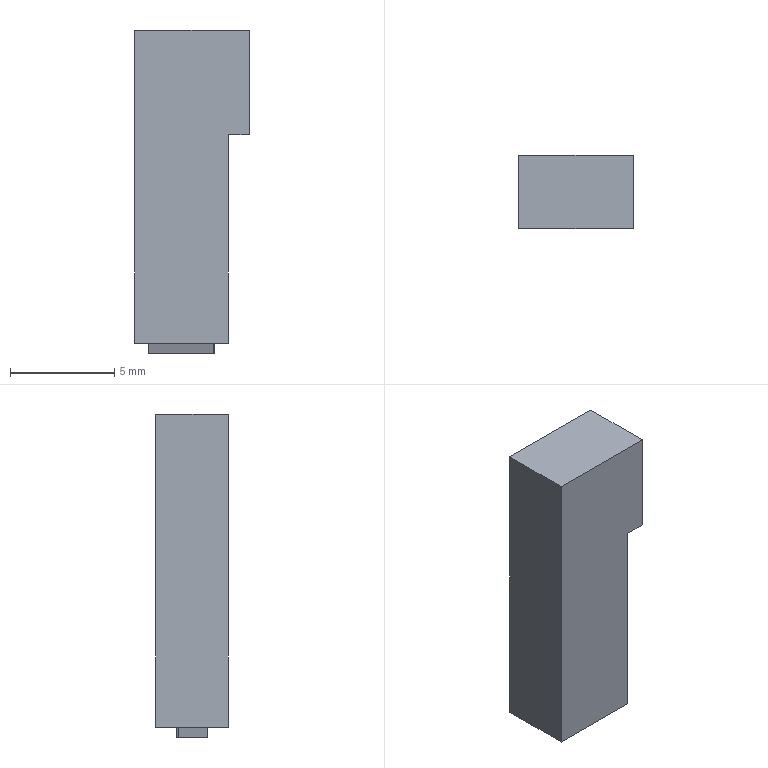Part | STEP file | gslz 2016.10.28-10_id1638_x_t | 1 solid | 13 faces | box 5.5 x 3.5 x 15.5 mm | volume 253.941 mm3 | plane 13
STEP:
#1=CARTESIAN_POINT('',(0.,0.,0.));
#2=DIRECTION('',(0.,0.,1.));
#3=DIRECTION('',(1.,0.,0.));
#4=AXIS2_PLACEMENT_3D('',#1,#2,#3);
#5=CARTESIAN_POINT('',(-688.56,94.749,15.));
#6=VERTEX_POINT('',#5);
#7=CARTESIAN_POINT('',(-694.06,94.749,15.));
#8=VERTEX_POINT('',#7);
#9=CARTESIAN_POINT('',(-691.31,94.749,15.));
#10=DIRECTION('',(-1.,0.000000055,0.));
#11=VECTOR('',#10,1.);
#12=LINE('',#9,#11);
#13=CARTESIAN_POINT('',(-694.06,94.749,15.));
#14=DIRECTION('',(-0.000000055,-1.,0.));
#15=DIRECTION('',(-1.,0.000000055,0.));
#16=AXIS2_PLACEMENT_3D('',#13,#14,#15);
#17=PLANE('',#16);
#18=CARTESIAN_POINT('',(-2.75,0.));
#19=DIRECTION('',(1.,0.));
#20=VECTOR('',#19,1.);
#21=LINE('',#18,#20);
#22=(GEOMETRIC_REPRESENTATION_CONTEXT(2)PARAMETRIC_REPRESENTATION_CONTEXT()REPRESENTATION_CONTEXT('',''));
#23=DEFINITIONAL_REPRESENTATION('',(#21),#22);
#24=PCURVE('',#17,#23);
#25=CARTESIAN_POINT('',(-694.06,96.499,15.));
#26=DIRECTION('',(0.,0.,1.));
#27=DIRECTION('',(1.,0.,0.));
#28=AXIS2_PLACEMENT_3D('',#25,#26,#27);
#29=PLANE('',#28);
#30=CARTESIAN_POINT('',(2.75,-1.75));
#31=DIRECTION('',(-1.,0.000000055));
#32=VECTOR('',#31,1.);
#33=LINE('',#30,#32);
#34=(GEOMETRIC_REPRESENTATION_CONTEXT(2)PARAMETRIC_REPRESENTATION_CONTEXT()REPRESENTATION_CONTEXT('',''));
#35=DEFINITIONAL_REPRESENTATION('',(#33),#34);
#36=PCURVE('',#29,#35);
#37=SURFACE_CURVE('',#12,(#24,#36),.PCURVE_S1.);
#38=EDGE_CURVE('',#6,#8,#37,.T.);
#39=ORIENTED_EDGE('',*,*,#38,.T.);
#40=CARTESIAN_POINT('',(-694.06,94.749,0.));
#41=VERTEX_POINT('',#40);
#42=CARTESIAN_POINT('',(-694.06,94.749,15.));
#43=DIRECTION('',(0.,0.,1.));
#44=VECTOR('',#43,1.);
#45=LINE('',#42,#44);
#46=CARTESIAN_POINT('',(0.,0.));
#47=DIRECTION('',(0.,-1.));
#48=VECTOR('',#47,1.);
#49=LINE('',#46,#48);
#50=(GEOMETRIC_REPRESENTATION_CONTEXT(2)PARAMETRIC_REPRESENTATION_CONTEXT()REPRESENTATION_CONTEXT('',''));
#51=DEFINITIONAL_REPRESENTATION('',(#49),#50);
#52=PCURVE('',#17,#51);
#53=CARTESIAN_POINT('',(-694.06,98.249,15.));
#54=DIRECTION('',(-1.,0.,0.));
#55=DIRECTION('',(0.,1.,0.));
#56=AXIS2_PLACEMENT_3D('',#53,#54,#55);
#57=PLANE('',#56);
#58=CARTESIAN_POINT('',(-3.5,0.));
#59=DIRECTION('',(0.,-1.));
#60=VECTOR('',#59,1.);
#61=LINE('',#58,#60);
#62=(GEOMETRIC_REPRESENTATION_CONTEXT(2)PARAMETRIC_REPRESENTATION_CONTEXT()REPRESENTATION_CONTEXT('',''));
#63=DEFINITIONAL_REPRESENTATION('',(#61),#62);
#64=PCURVE('',#57,#63);
#65=SURFACE_CURVE('',#45,(#52,#64),.PCURVE_S1.);
#66=EDGE_CURVE('',#41,#8,#65,.T.);
#67=ORIENTED_EDGE('',*,*,#66,.F.);
#68=CARTESIAN_POINT('',(-689.56,94.749,0.));
#69=VERTEX_POINT('',#68);
#70=CARTESIAN_POINT('',(-691.31,94.749,0.));
#71=DIRECTION('',(-1.,0.000000055,0.));
#72=VECTOR('',#71,1.);
#73=LINE('',#70,#72);
#74=CARTESIAN_POINT('',(-2.75,15.));
#75=DIRECTION('',(1.,0.));
#76=VECTOR('',#75,1.);
#77=LINE('',#74,#76);
#78=(GEOMETRIC_REPRESENTATION_CONTEXT(2)PARAMETRIC_REPRESENTATION_CONTEXT()REPRESENTATION_CONTEXT('',''));
#79=DEFINITIONAL_REPRESENTATION('',(#77),#78);
#80=PCURVE('',#17,#79);
#81=CARTESIAN_POINT('',(-694.06,96.499,0.));
#82=DIRECTION('',(0.,0.,1.));
#83=DIRECTION('',(1.,0.,0.));
#84=AXIS2_PLACEMENT_3D('',#81,#82,#83);
#85=PLANE('',#84);
#86=CARTESIAN_POINT('',(2.75,-1.75));
#87=DIRECTION('',(-1.,0.000000055));
#88=VECTOR('',#87,1.);
#89=LINE('',#86,#88);
#90=(GEOMETRIC_REPRESENTATION_CONTEXT(2)PARAMETRIC_REPRESENTATION_CONTEXT()REPRESENTATION_CONTEXT('',''));
#91=DEFINITIONAL_REPRESENTATION('',(#89),#90);
#92=PCURVE('',#85,#91);
#93=SURFACE_CURVE('',#73,(#80,#92),.PCURVE_S1.);
#94=EDGE_CURVE('',#69,#41,#93,.T.);
#95=ORIENTED_EDGE('',*,*,#94,.F.);
#96=CARTESIAN_POINT('',(-689.56,94.749,10.));
#97=VERTEX_POINT('',#96);
#98=CARTESIAN_POINT('',(-689.56,94.749,15.));
#99=DIRECTION('',(0.,0.,-1.));
#100=VECTOR('',#99,1.);
#101=LINE('',#98,#100);
#102=CARTESIAN_POINT('',(-4.5,0.));
#103=DIRECTION('',(0.,1.));
#104=VECTOR('',#103,1.);
#105=LINE('',#102,#104);
#106=(GEOMETRIC_REPRESENTATION_CONTEXT(2)PARAMETRIC_REPRESENTATION_CONTEXT()REPRESENTATION_CONTEXT('',''));
#107=DEFINITIONAL_REPRESENTATION('',(#105),#106);
#108=PCURVE('',#17,#107);
#109=CARTESIAN_POINT('',(-689.56,96.499,7.5));
#110=DIRECTION('',(1.,0.,0.));
#111=DIRECTION('',(0.,0.,-1.));
#112=AXIS2_PLACEMENT_3D('',#109,#110,#111);
#113=PLANE('',#112);
#114=CARTESIAN_POINT('',(-7.5,-1.75));
#115=DIRECTION('',(1.,0.));
#116=VECTOR('',#115,1.);
#117=LINE('',#114,#116);
#118=(GEOMETRIC_REPRESENTATION_CONTEXT(2)PARAMETRIC_REPRESENTATION_CONTEXT()REPRESENTATION_CONTEXT('',''));
#119=DEFINITIONAL_REPRESENTATION('',(#117),#118);
#120=PCURVE('',#113,#119);
#121=SURFACE_CURVE('',#101,(#108,#120),.PCURVE_S1.);
#122=EDGE_CURVE('',#97,#69,#121,.T.);
#123=ORIENTED_EDGE('',*,*,#122,.F.);
#124=CARTESIAN_POINT('',(-688.56,94.749,10.));
#125=VERTEX_POINT('',#124);
#126=CARTESIAN_POINT('',(-694.06,94.749,10.));
#127=DIRECTION('',(-1.,0.000000055,0.));
#128=VECTOR('',#127,1.);
#129=LINE('',#126,#128);
#130=CARTESIAN_POINT('',(0.,5.));
#131=DIRECTION('',(1.,0.));
#132=VECTOR('',#131,1.);
#133=LINE('',#130,#132);
#134=(GEOMETRIC_REPRESENTATION_CONTEXT(2)PARAMETRIC_REPRESENTATION_CONTEXT()REPRESENTATION_CONTEXT('',''));
#135=DEFINITIONAL_REPRESENTATION('',(#133),#134);
#136=PCURVE('',#17,#135);
#137=CARTESIAN_POINT('',(-694.06,96.499,10.));
#138=DIRECTION('',(0.,0.,1.));
#139=DIRECTION('',(1.,0.,0.));
#140=AXIS2_PLACEMENT_3D('',#137,#138,#139);
#141=PLANE('',#140);
#142=CARTESIAN_POINT('',(0.,-1.75));
#143=DIRECTION('',(-1.,0.000000055));
#144=VECTOR('',#143,1.);
#145=LINE('',#142,#144);
#146=(GEOMETRIC_REPRESENTATION_CONTEXT(2)PARAMETRIC_REPRESENTATION_CONTEXT()REPRESENTATION_CONTEXT('',''));
#147=DEFINITIONAL_REPRESENTATION('',(#145),#146);
#148=PCURVE('',#141,#147);
#149=SURFACE_CURVE('',#129,(#136,#148),.PCURVE_S1.);
#150=EDGE_CURVE('',#125,#97,#149,.T.);
#151=ORIENTED_EDGE('',*,*,#150,.F.);
#152=CARTESIAN_POINT('',(-688.56,94.749,15.));
#153=DIRECTION('',(0.,0.,1.));
#154=VECTOR('',#153,1.);
#155=LINE('',#152,#154);
#156=CARTESIAN_POINT('',(-5.5,0.));
#157=DIRECTION('',(0.,-1.));
#158=VECTOR('',#157,1.);
#159=LINE('',#156,#158);
#160=(GEOMETRIC_REPRESENTATION_CONTEXT(2)PARAMETRIC_REPRESENTATION_CONTEXT()REPRESENTATION_CONTEXT('',''));
#161=DEFINITIONAL_REPRESENTATION('',(#159),#160);
#162=PCURVE('',#17,#161);
#163=CARTESIAN_POINT('',(-688.56,94.749,15.));
#164=DIRECTION('',(1.,0.,0.));
#165=DIRECTION('',(0.,-1.,0.));
#166=AXIS2_PLACEMENT_3D('',#163,#164,#165);
#167=PLANE('',#166);
#168=CARTESIAN_POINT('',(0.,0.));
#169=DIRECTION('',(0.,-1.));
#170=VECTOR('',#169,1.);
#171=LINE('',#168,#170);
#172=(GEOMETRIC_REPRESENTATION_CONTEXT(2)PARAMETRIC_REPRESENTATION_CONTEXT()REPRESENTATION_CONTEXT('',''));
#173=DEFINITIONAL_REPRESENTATION('',(#171),#172);
#174=PCURVE('',#167,#173);
#175=SURFACE_CURVE('',#155,(#162,#174),.PCURVE_S1.);
#176=EDGE_CURVE('',#125,#6,#175,.T.);
#177=ORIENTED_EDGE('',*,*,#176,.T.);
#178=EDGE_LOOP('',(#39,#67,#95,#123,#151,#177));
#179=FACE_BOUND('',#178,.T.);
#180=ADVANCED_FACE('',(#179),#17,.T.);
#181=CARTESIAN_POINT('',(-694.06,98.249,0.));
#182=VERTEX_POINT('',#181);
#183=CARTESIAN_POINT('',(-689.56,98.249,0.));
#184=VERTEX_POINT('',#183);
#185=CARTESIAN_POINT('',(-691.31,98.249,0.));
#186=DIRECTION('',(1.,-0.000000055,0.));
#187=VECTOR('',#186,1.);
#188=LINE('',#185,#187);
#189=CARTESIAN_POINT('',(-688.56,98.249,15.));
#190=DIRECTION('',(0.000000055,1.,0.));
#191=DIRECTION('',(1.,-0.000000055,0.));
#192=AXIS2_PLACEMENT_3D('',#189,#190,#191);
#193=PLANE('',#192);
#194=CARTESIAN_POINT('',(-2.75,15.));
#195=DIRECTION('',(1.,0.));
#196=VECTOR('',#195,1.);
#197=LINE('',#194,#196);
#198=(GEOMETRIC_REPRESENTATION_CONTEXT(2)PARAMETRIC_REPRESENTATION_CONTEXT()REPRESENTATION_CONTEXT('',''));
#199=DEFINITIONAL_REPRESENTATION('',(#197),#198);
#200=PCURVE('',#193,#199);
#201=CARTESIAN_POINT('',(2.75,1.75));
#202=DIRECTION('',(1.,-0.000000055));
#203=VECTOR('',#202,1.);
#204=LINE('',#201,#203);
#205=(GEOMETRIC_REPRESENTATION_CONTEXT(2)PARAMETRIC_REPRESENTATION_CONTEXT()REPRESENTATION_CONTEXT('',''));
#206=DEFINITIONAL_REPRESENTATION('',(#204),#205);
#207=PCURVE('',#85,#206);
#208=SURFACE_CURVE('',#188,(#200,#207),.PCURVE_S1.);
#209=EDGE_CURVE('',#182,#184,#208,.T.);
#210=ORIENTED_EDGE('',*,*,#209,.F.);
#211=CARTESIAN_POINT('',(-694.06,98.249,15.));
#212=VERTEX_POINT('',#211);
#213=CARTESIAN_POINT('',(-694.06,98.249,15.));
#214=DIRECTION('',(0.,0.,1.));
#215=VECTOR('',#214,1.);
#216=LINE('',#213,#215);
#217=CARTESIAN_POINT('',(-5.5,0.));
#218=DIRECTION('',(0.,-1.));
#219=VECTOR('',#218,1.);
#220=LINE('',#217,#219);
#221=(GEOMETRIC_REPRESENTATION_CONTEXT(2)PARAMETRIC_REPRESENTATION_CONTEXT()REPRESENTATION_CONTEXT('',''));
#222=DEFINITIONAL_REPRESENTATION('',(#220),#221);
#223=PCURVE('',#193,#222);
#224=CARTESIAN_POINT('',(0.,0.));
#225=DIRECTION('',(0.,-1.));
#226=VECTOR('',#225,1.);
#227=LINE('',#224,#226);
#228=(GEOMETRIC_REPRESENTATION_CONTEXT(2)PARAMETRIC_REPRESENTATION_CONTEXT()REPRESENTATION_CONTEXT('',''));
#229=DEFINITIONAL_REPRESENTATION('',(#227),#228);
#230=PCURVE('',#57,#229);
#231=SURFACE_CURVE('',#216,(#223,#230),.PCURVE_S1.);
#232=EDGE_CURVE('',#182,#212,#231,.T.);
#233=ORIENTED_EDGE('',*,*,#232,.T.);
#234=CARTESIAN_POINT('',(-688.56,98.249,15.));
#235=VERTEX_POINT('',#234);
#236=CARTESIAN_POINT('',(-691.31,98.249,15.));
#237=DIRECTION('',(1.,-0.000000055,0.));
#238=VECTOR('',#237,1.);
#239=LINE('',#236,#238);
#240=CARTESIAN_POINT('',(-2.75,0.));
#241=DIRECTION('',(1.,0.));
#242=VECTOR('',#241,1.);
#243=LINE('',#240,#242);
#244=(GEOMETRIC_REPRESENTATION_CONTEXT(2)PARAMETRIC_REPRESENTATION_CONTEXT()REPRESENTATION_CONTEXT('',''));
#245=DEFINITIONAL_REPRESENTATION('',(#243),#244);
#246=PCURVE('',#193,#245);
#247=CARTESIAN_POINT('',(2.75,1.75));
#248=DIRECTION('',(1.,-0.000000055));
#249=VECTOR('',#248,1.);
#250=LINE('',#247,#249);
#251=(GEOMETRIC_REPRESENTATION_CONTEXT(2)PARAMETRIC_REPRESENTATION_CONTEXT()REPRESENTATION_CONTEXT('',''));
#252=DEFINITIONAL_REPRESENTATION('',(#250),#251);
#253=PCURVE('',#29,#252);
#254=SURFACE_CURVE('',#239,(#246,#253),.PCURVE_S1.);
#255=EDGE_CURVE('',#212,#235,#254,.T.);
#256=ORIENTED_EDGE('',*,*,#255,.T.);
#257=CARTESIAN_POINT('',(-688.56,98.249,10.));
#258=VERTEX_POINT('',#257);
#259=CARTESIAN_POINT('',(-688.56,98.249,15.));
#260=DIRECTION('',(0.,0.,1.));
#261=VECTOR('',#260,1.);
#262=LINE('',#259,#261);
#263=CARTESIAN_POINT('',(0.,0.));
#264=DIRECTION('',(0.,-1.));
#265=VECTOR('',#264,1.);
#266=LINE('',#263,#265);
#267=(GEOMETRIC_REPRESENTATION_CONTEXT(2)PARAMETRIC_REPRESENTATION_CONTEXT()REPRESENTATION_CONTEXT('',''));
#268=DEFINITIONAL_REPRESENTATION('',(#266),#267);
#269=PCURVE('',#193,#268);
#270=CARTESIAN_POINT('',(-3.5,0.));
#271=DIRECTION('',(0.,-1.));
#272=VECTOR('',#271,1.);
#273=LINE('',#270,#272);
#274=(GEOMETRIC_REPRESENTATION_CONTEXT(2)PARAMETRIC_REPRESENTATION_CONTEXT()REPRESENTATION_CONTEXT('',''));
#275=DEFINITIONAL_REPRESENTATION('',(#273),#274);
#276=PCURVE('',#167,#275);
#277=SURFACE_CURVE('',#262,(#269,#276),.PCURVE_S1.);
#278=EDGE_CURVE('',#258,#235,#277,.T.);
#279=ORIENTED_EDGE('',*,*,#278,.F.);
#280=CARTESIAN_POINT('',(-689.56,98.249,10.));
#281=VERTEX_POINT('',#280);
#282=CARTESIAN_POINT('',(-688.56,98.249,10.));
#283=DIRECTION('',(1.,-0.000000055,0.));
#284=VECTOR('',#283,1.);
#285=LINE('',#282,#284);
#286=CARTESIAN_POINT('',(0.,5.));
#287=DIRECTION('',(1.,0.));
#288=VECTOR('',#287,1.);
#289=LINE('',#286,#288);
#290=(GEOMETRIC_REPRESENTATION_CONTEXT(2)PARAMETRIC_REPRESENTATION_CONTEXT()REPRESENTATION_CONTEXT('',''));
#291=DEFINITIONAL_REPRESENTATION('',(#289),#290);
#292=PCURVE('',#193,#291);
#293=CARTESIAN_POINT('',(5.5,1.75));
#294=DIRECTION('',(1.,-0.000000055));
#295=VECTOR('',#294,1.);
#296=LINE('',#293,#295);
#297=(GEOMETRIC_REPRESENTATION_CONTEXT(2)PARAMETRIC_REPRESENTATION_CONTEXT()REPRESENTATION_CONTEXT('',''));
#298=DEFINITIONAL_REPRESENTATION('',(#296),#297);
#299=PCURVE('',#141,#298);
#300=SURFACE_CURVE('',#285,(#292,#299),.PCURVE_S1.);
#301=EDGE_CURVE('',#281,#258,#300,.T.);
#302=ORIENTED_EDGE('',*,*,#301,.F.);
#303=CARTESIAN_POINT('',(-689.56,98.249,15.));
#304=DIRECTION('',(0.,0.,1.));
#305=VECTOR('',#304,1.);
#306=LINE('',#303,#305);
#307=CARTESIAN_POINT('',(-1.,0.));
#308=DIRECTION('',(0.,-1.));
#309=VECTOR('',#308,1.);
#310=LINE('',#307,#309);
#311=(GEOMETRIC_REPRESENTATION_CONTEXT(2)PARAMETRIC_REPRESENTATION_CONTEXT()REPRESENTATION_CONTEXT('',''));
#312=DEFINITIONAL_REPRESENTATION('',(#310),#311);
#313=PCURVE('',#193,#312);
#314=CARTESIAN_POINT('',(-7.5,1.75));
#315=DIRECTION('',(-1.,0.));
#316=VECTOR('',#315,1.);
#317=LINE('',#314,#316);
#318=(GEOMETRIC_REPRESENTATION_CONTEXT(2)PARAMETRIC_REPRESENTATION_CONTEXT()REPRESENTATION_CONTEXT('',''));
#319=DEFINITIONAL_REPRESENTATION('',(#317),#318);
#320=PCURVE('',#113,#319);
#321=SURFACE_CURVE('',#306,(#313,#320),.PCURVE_S1.);
#322=EDGE_CURVE('',#184,#281,#321,.T.);
#323=ORIENTED_EDGE('',*,*,#322,.F.);
#324=EDGE_LOOP('',(#210,#233,#256,#279,#302,#323));
#325=FACE_BOUND('',#324,.T.);
#326=ADVANCED_FACE('',(#325),#193,.T.);
#327=ORIENTED_EDGE('',*,*,#255,.F.);
#328=CARTESIAN_POINT('',(-694.06,96.499,15.));
#329=DIRECTION('',(0.,1.,0.));
#330=VECTOR('',#329,1.);
#331=LINE('',#328,#330);
#332=CARTESIAN_POINT('',(0.,0.));
#333=DIRECTION('',(0.,1.));
#334=VECTOR('',#333,1.);
#335=LINE('',#332,#334);
#336=(GEOMETRIC_REPRESENTATION_CONTEXT(2)PARAMETRIC_REPRESENTATION_CONTEXT()REPRESENTATION_CONTEXT('',''));
#337=DEFINITIONAL_REPRESENTATION('',(#335),#336);
#338=PCURVE('',#29,#337);
#339=CARTESIAN_POINT('',(-1.75,0.));
#340=DIRECTION('',(1.,0.));
#341=VECTOR('',#340,1.);
#342=LINE('',#339,#341);
#343=(GEOMETRIC_REPRESENTATION_CONTEXT(2)PARAMETRIC_REPRESENTATION_CONTEXT()REPRESENTATION_CONTEXT('',''));
#344=DEFINITIONAL_REPRESENTATION('',(#342),#343);
#345=PCURVE('',#57,#344);
#346=SURFACE_CURVE('',#331,(#338,#345),.PCURVE_S1.);
#347=EDGE_CURVE('',#8,#212,#346,.T.);
#348=ORIENTED_EDGE('',*,*,#347,.F.);
#349=ORIENTED_EDGE('',*,*,#38,.F.);
#350=CARTESIAN_POINT('',(-688.56,96.499,15.));
#351=DIRECTION('',(0.,-1.,0.));
#352=VECTOR('',#351,1.);
#353=LINE('',#350,#352);
#354=CARTESIAN_POINT('',(5.5,-0.000000303));
#355=DIRECTION('',(0.,-1.));
#356=VECTOR('',#355,1.);
#357=LINE('',#354,#356);
#358=(GEOMETRIC_REPRESENTATION_CONTEXT(2)PARAMETRIC_REPRESENTATION_CONTEXT()REPRESENTATION_CONTEXT('',''));
#359=DEFINITIONAL_REPRESENTATION('',(#357),#358);
#360=PCURVE('',#29,#359);
#361=CARTESIAN_POINT('',(-1.75,0.));
#362=DIRECTION('',(1.,0.));
#363=VECTOR('',#362,1.);
#364=LINE('',#361,#363);
#365=(GEOMETRIC_REPRESENTATION_CONTEXT(2)PARAMETRIC_REPRESENTATION_CONTEXT()REPRESENTATION_CONTEXT('',''));
#366=DEFINITIONAL_REPRESENTATION('',(#364),#365);
#367=PCURVE('',#167,#366);
#368=SURFACE_CURVE('',#353,(#360,#367),.PCURVE_S1.);
#369=EDGE_CURVE('',#235,#6,#368,.T.);
#370=ORIENTED_EDGE('',*,*,#369,.F.);
#371=EDGE_LOOP('',(#327,#348,#349,#370));
#372=FACE_BOUND('',#371,.T.);
#373=ADVANCED_FACE('',(#372),#29,.T.);
#374=CARTESIAN_POINT('',(-693.353,97.249,0.));
#375=VERTEX_POINT('',#374);
#376=CARTESIAN_POINT('',(-693.411,97.153,0.));
#377=VERTEX_POINT('',#376);
#378=CARTESIAN_POINT('',(-693.875,96.387,0.));
#379=DIRECTION('',(-0.5182,-0.8552,0.));
#380=VECTOR('',#379,1.);
#381=LINE('',#378,#380);
#382=CARTESIAN_POINT('',(0.185,-0.1121));
#383=DIRECTION('',(-0.5182,-0.8552));
#384=VECTOR('',#383,1.);
#385=LINE('',#382,#384);
#386=(GEOMETRIC_REPRESENTATION_CONTEXT(2)PARAMETRIC_REPRESENTATION_CONTEXT()REPRESENTATION_CONTEXT('',''));
#387=DEFINITIONAL_REPRESENTATION('',(#385),#386);
#388=PCURVE('',#85,#387);
#389=CARTESIAN_POINT('',(-693.411,97.153,-0.5));
#390=DIRECTION('',(-0.8552,0.5182,0.));
#391=DIRECTION('',(0.5182,0.8552,0.));
#392=AXIS2_PLACEMENT_3D('',#389,#390,#391);
#393=PLANE('',#392);
#394=CARTESIAN_POINT('',(-0.8956,-0.5));
#395=DIRECTION('',(-1.,0.));
#396=VECTOR('',#395,1.);
#397=LINE('',#394,#396);
#398=(GEOMETRIC_REPRESENTATION_CONTEXT(2)PARAMETRIC_REPRESENTATION_CONTEXT()REPRESENTATION_CONTEXT('',''));
#399=DEFINITIONAL_REPRESENTATION('',(#397),#398);
#400=PCURVE('',#393,#399);
#401=SURFACE_CURVE('',#381,(#388,#400),.PCURVE_S1.);
#402=EDGE_CURVE('',#375,#377,#401,.T.);
#403=ORIENTED_EDGE('',*,*,#402,.T.);
#404=CARTESIAN_POINT('',(-690.282,95.749,0.));
#405=VERTEX_POINT('',#404);
#406=CARTESIAN_POINT('',(-693.707,97.286,0.));
#407=DIRECTION('',(0.9123,-0.4094,0.));
#408=VECTOR('',#407,1.);
#409=LINE('',#406,#408);
#410=CARTESIAN_POINT('',(0.353,0.7867));
#411=DIRECTION('',(0.9123,-0.4094));
#412=VECTOR('',#411,1.);
#413=LINE('',#410,#412);
#414=(GEOMETRIC_REPRESENTATION_CONTEXT(2)PARAMETRIC_REPRESENTATION_CONTEXT()REPRESENTATION_CONTEXT('',''));
#415=DEFINITIONAL_REPRESENTATION('',(#413),#414);
#416=PCURVE('',#85,#415);
#417=CARTESIAN_POINT('',(-690.282,95.749,-0.5));
#418=DIRECTION('',(-0.4094,-0.9123,0.));
#419=DIRECTION('',(-0.9123,0.4094,0.));
#420=AXIS2_PLACEMENT_3D('',#417,#418,#419);
#421=PLANE('',#420);
#422=CARTESIAN_POINT('',(3.754,-0.5));
#423=DIRECTION('',(-1.,0.));
#424=VECTOR('',#423,1.);
#425=LINE('',#422,#424);
#426=(GEOMETRIC_REPRESENTATION_CONTEXT(2)PARAMETRIC_REPRESENTATION_CONTEXT()REPRESENTATION_CONTEXT('',''));
#427=DEFINITIONAL_REPRESENTATION('',(#425),#426);
#428=PCURVE('',#421,#427);
#429=SURFACE_CURVE('',#409,(#416,#428),.PCURVE_S1.);
#430=EDGE_CURVE('',#377,#405,#429,.T.);
#431=ORIENTED_EDGE('',*,*,#430,.T.);
#432=CARTESIAN_POINT('',(-690.224,95.845,0.));
#433=VERTEX_POINT('',#432);
#434=CARTESIAN_POINT('',(-690.965,94.623,0.));
#435=DIRECTION('',(0.5182,0.8552,0.));
#436=VECTOR('',#435,1.);
#437=LINE('',#434,#436);
#438=CARTESIAN_POINT('',(3.095,-1.876));
#439=DIRECTION('',(0.5182,0.8552));
#440=VECTOR('',#439,1.);
#441=LINE('',#438,#440);
#442=(GEOMETRIC_REPRESENTATION_CONTEXT(2)PARAMETRIC_REPRESENTATION_CONTEXT()REPRESENTATION_CONTEXT('',''));
#443=DEFINITIONAL_REPRESENTATION('',(#441),#442);
#444=PCURVE('',#85,#443);
#445=CARTESIAN_POINT('',(-690.224,95.845,-0.5));
#446=DIRECTION('',(0.8552,-0.5182,0.));
#447=DIRECTION('',(-0.5182,-0.8552,0.));
#448=AXIS2_PLACEMENT_3D('',#445,#446,#447);
#449=PLANE('',#448);
#450=CARTESIAN_POINT('',(1.429,-0.5));
#451=DIRECTION('',(-1.,0.));
#452=VECTOR('',#451,1.);
#453=LINE('',#450,#452);
#454=(GEOMETRIC_REPRESENTATION_CONTEXT(2)PARAMETRIC_REPRESENTATION_CONTEXT()REPRESENTATION_CONTEXT('',''));
#455=DEFINITIONAL_REPRESENTATION('',(#453),#454);
#456=PCURVE('',#449,#455);
#457=SURFACE_CURVE('',#437,(#444,#456),.PCURVE_S1.);
#458=EDGE_CURVE('',#405,#433,#457,.T.);
#459=ORIENTED_EDGE('',*,*,#458,.T.);
#460=CARTESIAN_POINT('',(-693.661,97.388,0.));
#461=DIRECTION('',(-0.9123,0.4094,0.));
#462=VECTOR('',#461,1.);
#463=LINE('',#460,#462);
#464=CARTESIAN_POINT('',(0.3987,0.8885));
#465=DIRECTION('',(-0.9123,0.4094));
#466=VECTOR('',#465,1.);
#467=LINE('',#464,#466);
#468=(GEOMETRIC_REPRESENTATION_CONTEXT(2)PARAMETRIC_REPRESENTATION_CONTEXT()REPRESENTATION_CONTEXT('',''));
#469=DEFINITIONAL_REPRESENTATION('',(#467),#468);
#470=PCURVE('',#85,#469);
#471=CARTESIAN_POINT('',(-693.353,97.249,-0.5));
#472=DIRECTION('',(0.4094,0.9123,0.));
#473=DIRECTION('',(0.9123,-0.4094,0.));
#474=AXIS2_PLACEMENT_3D('',#471,#472,#473);
#475=PLANE('',#474);
#476=CARTESIAN_POINT('',(-0.3383,-0.5));
#477=DIRECTION('',(-1.,0.));
#478=VECTOR('',#477,1.);
#479=LINE('',#476,#478);
#480=(GEOMETRIC_REPRESENTATION_CONTEXT(2)PARAMETRIC_REPRESENTATION_CONTEXT()REPRESENTATION_CONTEXT('',''));
#481=DEFINITIONAL_REPRESENTATION('',(#479),#480);
#482=PCURVE('',#475,#481);
#483=SURFACE_CURVE('',#463,(#470,#482),.PCURVE_S1.);
#484=EDGE_CURVE('',#433,#375,#483,.T.);
#485=ORIENTED_EDGE('',*,*,#484,.T.);
#486=EDGE_LOOP('',(#403,#431,#459,#485));
#487=FACE_BOUND('',#486,.T.);
#488=CARTESIAN_POINT('',(-689.56,96.499,0.));
#489=DIRECTION('',(0.,-1.,0.));
#490=VECTOR('',#489,1.);
#491=LINE('',#488,#490);
#492=CARTESIAN_POINT('',(4.5,0.));
#493=DIRECTION('',(0.,-1.));
#494=VECTOR('',#493,1.);
#495=LINE('',#492,#494);
#496=(GEOMETRIC_REPRESENTATION_CONTEXT(2)PARAMETRIC_REPRESENTATION_CONTEXT()REPRESENTATION_CONTEXT('',''));
#497=DEFINITIONAL_REPRESENTATION('',(#495),#496);
#498=PCURVE('',#85,#497);
#499=CARTESIAN_POINT('',(7.5,0.000000303));
#500=DIRECTION('',(0.,-1.));
#501=VECTOR('',#500,1.);
#502=LINE('',#499,#501);
#503=(GEOMETRIC_REPRESENTATION_CONTEXT(2)PARAMETRIC_REPRESENTATION_CONTEXT()REPRESENTATION_CONTEXT('',''));
#504=DEFINITIONAL_REPRESENTATION('',(#502),#503);
#505=PCURVE('',#113,#504);
#506=SURFACE_CURVE('',#491,(#498,#505),.PCURVE_S1.);
#507=EDGE_CURVE('',#184,#69,#506,.T.);
#508=ORIENTED_EDGE('',*,*,#507,.T.);
#509=ORIENTED_EDGE('',*,*,#94,.T.);
#510=CARTESIAN_POINT('',(-694.06,96.499,0.));
#511=DIRECTION('',(0.,1.,0.));
#512=VECTOR('',#511,1.);
#513=LINE('',#510,#512);
#514=CARTESIAN_POINT('',(0.,0.));
#515=DIRECTION('',(0.,1.));
#516=VECTOR('',#515,1.);
#517=LINE('',#514,#516);
#518=(GEOMETRIC_REPRESENTATION_CONTEXT(2)PARAMETRIC_REPRESENTATION_CONTEXT()REPRESENTATION_CONTEXT('',''));
#519=DEFINITIONAL_REPRESENTATION('',(#517),#518);
#520=PCURVE('',#85,#519);
#521=CARTESIAN_POINT('',(-1.75,15.));
#522=DIRECTION('',(1.,0.));
#523=VECTOR('',#522,1.);
#524=LINE('',#521,#523);
#525=(GEOMETRIC_REPRESENTATION_CONTEXT(2)PARAMETRIC_REPRESENTATION_CONTEXT()REPRESENTATION_CONTEXT('',''));
#526=DEFINITIONAL_REPRESENTATION('',(#524),#525);
#527=PCURVE('',#57,#526);
#528=SURFACE_CURVE('',#513,(#520,#527),.PCURVE_S1.);
#529=EDGE_CURVE('',#41,#182,#528,.T.);
#530=ORIENTED_EDGE('',*,*,#529,.T.);
#531=ORIENTED_EDGE('',*,*,#209,.T.);
#532=EDGE_LOOP('',(#508,#509,#530,#531));
#533=FACE_BOUND('',#532,.T.);
#534=ADVANCED_FACE('',(#487,#533),#85,.F.);
#535=ORIENTED_EDGE('',*,*,#529,.F.);
#536=ORIENTED_EDGE('',*,*,#66,.T.);
#537=ORIENTED_EDGE('',*,*,#347,.T.);
#538=ORIENTED_EDGE('',*,*,#232,.F.);
#539=EDGE_LOOP('',(#535,#536,#537,#538));
#540=FACE_BOUND('',#539,.T.);
#541=ADVANCED_FACE('',(#540),#57,.T.);
#542=CARTESIAN_POINT('',(-689.56,96.499,10.));
#543=DIRECTION('',(0.,1.,0.));
#544=VECTOR('',#543,1.);
#545=LINE('',#542,#544);
#546=CARTESIAN_POINT('',(-2.5,0.000000303));
#547=DIRECTION('',(0.,1.));
#548=VECTOR('',#547,1.);
#549=LINE('',#546,#548);
#550=(GEOMETRIC_REPRESENTATION_CONTEXT(2)PARAMETRIC_REPRESENTATION_CONTEXT()REPRESENTATION_CONTEXT('',''));
#551=DEFINITIONAL_REPRESENTATION('',(#549),#550);
#552=PCURVE('',#113,#551);
#553=CARTESIAN_POINT('',(4.5,0.));
#554=DIRECTION('',(0.,1.));
#555=VECTOR('',#554,1.);
#556=LINE('',#553,#555);
#557=(GEOMETRIC_REPRESENTATION_CONTEXT(2)PARAMETRIC_REPRESENTATION_CONTEXT()REPRESENTATION_CONTEXT('',''));
#558=DEFINITIONAL_REPRESENTATION('',(#556),#557);
#559=PCURVE('',#141,#558);
#560=SURFACE_CURVE('',#545,(#552,#559),.PCURVE_S1.);
#561=EDGE_CURVE('',#97,#281,#560,.T.);
#562=ORIENTED_EDGE('',*,*,#561,.F.);
#563=ORIENTED_EDGE('',*,*,#122,.T.);
#564=ORIENTED_EDGE('',*,*,#507,.F.);
#565=ORIENTED_EDGE('',*,*,#322,.T.);
#566=EDGE_LOOP('',(#562,#563,#564,#565));
#567=FACE_BOUND('',#566,.T.);
#568=ADVANCED_FACE('',(#567),#113,.T.);
#569=CARTESIAN_POINT('',(-688.56,94.749,10.));
#570=DIRECTION('',(0.,-1.,0.));
#571=VECTOR('',#570,1.);
#572=LINE('',#569,#571);
#573=CARTESIAN_POINT('',(0.,5.));
#574=DIRECTION('',(1.,0.));
#575=VECTOR('',#574,1.);
#576=LINE('',#573,#575);
#577=(GEOMETRIC_REPRESENTATION_CONTEXT(2)PARAMETRIC_REPRESENTATION_CONTEXT()REPRESENTATION_CONTEXT('',''));
#578=DEFINITIONAL_REPRESENTATION('',(#576),#577);
#579=PCURVE('',#167,#578);
#580=CARTESIAN_POINT('',(5.5,-1.75));
#581=DIRECTION('',(0.,-1.));
#582=VECTOR('',#581,1.);
#583=LINE('',#580,#582);
#584=(GEOMETRIC_REPRESENTATION_CONTEXT(2)PARAMETRIC_REPRESENTATION_CONTEXT()REPRESENTATION_CONTEXT('',''));
#585=DEFINITIONAL_REPRESENTATION('',(#583),#584);
#586=PCURVE('',#141,#585);
#587=SURFACE_CURVE('',#572,(#579,#586),.PCURVE_S1.);
#588=EDGE_CURVE('',#258,#125,#587,.T.);
#589=ORIENTED_EDGE('',*,*,#588,.F.);
#590=ORIENTED_EDGE('',*,*,#278,.T.);
#591=ORIENTED_EDGE('',*,*,#369,.T.);
#592=ORIENTED_EDGE('',*,*,#176,.F.);
#593=EDGE_LOOP('',(#589,#590,#591,#592));
#594=FACE_BOUND('',#593,.T.);
#595=ADVANCED_FACE('',(#594),#167,.T.);
#596=ORIENTED_EDGE('',*,*,#301,.T.);
#597=ORIENTED_EDGE('',*,*,#588,.T.);
#598=ORIENTED_EDGE('',*,*,#150,.T.);
#599=ORIENTED_EDGE('',*,*,#561,.T.);
#600=EDGE_LOOP('',(#596,#597,#598,#599));
#601=FACE_BOUND('',#600,.T.);
#602=ADVANCED_FACE('',(#601),#141,.F.);
#603=ORIENTED_EDGE('',*,*,#484,.F.);
#604=CARTESIAN_POINT('',(-690.224,95.845,-0.5));
#605=VERTEX_POINT('',#604);
#606=CARTESIAN_POINT('',(-690.224,95.845,-0.5));
#607=DIRECTION('',(0.,0.,-1.));
#608=VECTOR('',#607,1.);
#609=LINE('',#606,#608);
#610=CARTESIAN_POINT('',(3.429,0.));
#611=DIRECTION('',(0.,1.));
#612=VECTOR('',#611,1.);
#613=LINE('',#610,#612);
#614=(GEOMETRIC_REPRESENTATION_CONTEXT(2)PARAMETRIC_REPRESENTATION_CONTEXT()REPRESENTATION_CONTEXT('',''));
#615=DEFINITIONAL_REPRESENTATION('',(#613),#614);
#616=PCURVE('',#475,#615);
#617=CARTESIAN_POINT('',(0.,0.));
#618=DIRECTION('',(0.,1.));
#619=VECTOR('',#618,1.);
#620=LINE('',#617,#619);
#621=(GEOMETRIC_REPRESENTATION_CONTEXT(2)PARAMETRIC_REPRESENTATION_CONTEXT()REPRESENTATION_CONTEXT('',''));
#622=DEFINITIONAL_REPRESENTATION('',(#620),#621);
#623=PCURVE('',#449,#622);
#624=SURFACE_CURVE('',#609,(#616,#623),.PCURVE_S1.);
#625=EDGE_CURVE('',#433,#605,#624,.T.);
#626=ORIENTED_EDGE('',*,*,#625,.T.);
#627=CARTESIAN_POINT('',(-693.353,97.249,-0.5));
#628=VERTEX_POINT('',#627);
#629=CARTESIAN_POINT('',(-691.788,96.547,-0.5));
#630=DIRECTION('',(-0.9123,0.4094,0.));
#631=VECTOR('',#630,1.);
#632=LINE('',#629,#631);
#633=CARTESIAN_POINT('',(1.714,0.));
#634=DIRECTION('',(-1.,0.));
#635=VECTOR('',#634,1.);
#636=LINE('',#633,#635);
#637=(GEOMETRIC_REPRESENTATION_CONTEXT(2)PARAMETRIC_REPRESENTATION_CONTEXT()REPRESENTATION_CONTEXT('',''));
#638=DEFINITIONAL_REPRESENTATION('',(#636),#637);
#639=PCURVE('',#475,#638);
#640=CARTESIAN_POINT('',(-691.788,96.547,-0.5));
#641=DIRECTION('',(0.,0.,-1.));
#642=DIRECTION('',(-1.,0.,0.));
#643=AXIS2_PLACEMENT_3D('',#640,#641,#642);
#644=PLANE('',#643);
#645=CARTESIAN_POINT('',(0.,0.));
#646=DIRECTION('',(0.9123,0.4094));
#647=VECTOR('',#646,1.);
#648=LINE('',#645,#647);
#649=(GEOMETRIC_REPRESENTATION_CONTEXT(2)PARAMETRIC_REPRESENTATION_CONTEXT()REPRESENTATION_CONTEXT('',''));
#650=DEFINITIONAL_REPRESENTATION('',(#648),#649);
#651=PCURVE('',#644,#650);
#652=SURFACE_CURVE('',#632,(#639,#651),.PCURVE_S1.);
#653=EDGE_CURVE('',#605,#628,#652,.T.);
#654=ORIENTED_EDGE('',*,*,#653,.T.);
#655=CARTESIAN_POINT('',(-693.353,97.249,-0.5));
#656=DIRECTION('',(0.,0.,-1.));
#657=VECTOR('',#656,1.);
#658=LINE('',#655,#657);
#659=CARTESIAN_POINT('',(0.,0.));
#660=DIRECTION('',(0.,1.));
#661=VECTOR('',#660,1.);
#662=LINE('',#659,#661);
#663=(GEOMETRIC_REPRESENTATION_CONTEXT(2)PARAMETRIC_REPRESENTATION_CONTEXT()REPRESENTATION_CONTEXT('',''));
#664=DEFINITIONAL_REPRESENTATION('',(#662),#663);
#665=PCURVE('',#475,#664);
#666=CARTESIAN_POINT('',(0.1124,0.));
#667=DIRECTION('',(0.,1.));
#668=VECTOR('',#667,1.);
#669=LINE('',#666,#668);
#670=(GEOMETRIC_REPRESENTATION_CONTEXT(2)PARAMETRIC_REPRESENTATION_CONTEXT()REPRESENTATION_CONTEXT('',''));
#671=DEFINITIONAL_REPRESENTATION('',(#669),#670);
#672=PCURVE('',#393,#671);
#673=SURFACE_CURVE('',#658,(#665,#672),.PCURVE_S1.);
#674=EDGE_CURVE('',#375,#628,#673,.T.);
#675=ORIENTED_EDGE('',*,*,#674,.F.);
#676=EDGE_LOOP('',(#603,#626,#654,#675));
#677=FACE_BOUND('',#676,.T.);
#678=ADVANCED_FACE('',(#677),#475,.T.);
#679=ORIENTED_EDGE('',*,*,#458,.F.);
#680=CARTESIAN_POINT('',(-690.282,95.749,-0.5));
#681=VERTEX_POINT('',#680);
#682=CARTESIAN_POINT('',(-690.282,95.749,-0.5));
#683=DIRECTION('',(0.,0.,-1.));
#684=VECTOR('',#683,1.);
#685=LINE('',#682,#684);
#686=CARTESIAN_POINT('',(0.1124,0.));
#687=DIRECTION('',(0.,1.));
#688=VECTOR('',#687,1.);
#689=LINE('',#686,#688);
#690=(GEOMETRIC_REPRESENTATION_CONTEXT(2)PARAMETRIC_REPRESENTATION_CONTEXT()REPRESENTATION_CONTEXT('',''));
#691=DEFINITIONAL_REPRESENTATION('',(#689),#690);
#692=PCURVE('',#449,#691);
#693=CARTESIAN_POINT('',(0.,0.));
#694=DIRECTION('',(0.,1.));
#695=VECTOR('',#694,1.);
#696=LINE('',#693,#695);
#697=(GEOMETRIC_REPRESENTATION_CONTEXT(2)PARAMETRIC_REPRESENTATION_CONTEXT()REPRESENTATION_CONTEXT('',''));
#698=DEFINITIONAL_REPRESENTATION('',(#696),#697);
#699=PCURVE('',#421,#698);
#700=SURFACE_CURVE('',#685,(#692,#699),.PCURVE_S1.);
#701=EDGE_CURVE('',#405,#681,#700,.T.);
#702=ORIENTED_EDGE('',*,*,#701,.T.);
#703=CARTESIAN_POINT('',(-690.253,95.797,-0.5));
#704=DIRECTION('',(0.5182,0.8552,0.));
#705=VECTOR('',#704,1.);
#706=LINE('',#703,#705);
#707=CARTESIAN_POINT('',(0.0562,0.));
#708=DIRECTION('',(-1.,0.));
#709=VECTOR('',#708,1.);
#710=LINE('',#707,#709);
#711=(GEOMETRIC_REPRESENTATION_CONTEXT(2)PARAMETRIC_REPRESENTATION_CONTEXT()REPRESENTATION_CONTEXT('',''));
#712=DEFINITIONAL_REPRESENTATION('',(#710),#711);
#713=PCURVE('',#449,#712);
#714=CARTESIAN_POINT('',(-1.535,-0.75));
#715=DIRECTION('',(-0.5182,0.8552));
#716=VECTOR('',#715,1.);
#717=LINE('',#714,#716);
#718=(GEOMETRIC_REPRESENTATION_CONTEXT(2)PARAMETRIC_REPRESENTATION_CONTEXT()REPRESENTATION_CONTEXT('',''));
#719=DEFINITIONAL_REPRESENTATION('',(#717),#718);
#720=PCURVE('',#644,#719);
#721=SURFACE_CURVE('',#706,(#713,#720),.PCURVE_S1.);
#722=EDGE_CURVE('',#681,#605,#721,.T.);
#723=ORIENTED_EDGE('',*,*,#722,.T.);
#724=ORIENTED_EDGE('',*,*,#625,.F.);
#725=EDGE_LOOP('',(#679,#702,#723,#724));
#726=FACE_BOUND('',#725,.T.);
#727=ADVANCED_FACE('',(#726),#449,.T.);
#728=ORIENTED_EDGE('',*,*,#430,.F.);
#729=CARTESIAN_POINT('',(-693.411,97.153,-0.5));
#730=VERTEX_POINT('',#729);
#731=CARTESIAN_POINT('',(-693.411,97.153,-0.5));
#732=DIRECTION('',(0.,0.,-1.));
#733=VECTOR('',#732,1.);
#734=LINE('',#731,#733);
#735=CARTESIAN_POINT('',(3.429,0.));
#736=DIRECTION('',(0.,1.));
#737=VECTOR('',#736,1.);
#738=LINE('',#735,#737);
#739=(GEOMETRIC_REPRESENTATION_CONTEXT(2)PARAMETRIC_REPRESENTATION_CONTEXT()REPRESENTATION_CONTEXT('',''));
#740=DEFINITIONAL_REPRESENTATION('',(#738),#739);
#741=PCURVE('',#421,#740);
#742=CARTESIAN_POINT('',(0.,0.));
#743=DIRECTION('',(0.,1.));
#744=VECTOR('',#743,1.);
#745=LINE('',#742,#744);
#746=(GEOMETRIC_REPRESENTATION_CONTEXT(2)PARAMETRIC_REPRESENTATION_CONTEXT()REPRESENTATION_CONTEXT('',''));
#747=DEFINITIONAL_REPRESENTATION('',(#745),#746);
#748=PCURVE('',#393,#747);
#749=SURFACE_CURVE('',#734,(#741,#748),.PCURVE_S1.);
#750=EDGE_CURVE('',#377,#730,#749,.T.);
#751=ORIENTED_EDGE('',*,*,#750,.T.);
#752=CARTESIAN_POINT('',(-691.847,96.451,-0.5));
#753=DIRECTION('',(0.9123,-0.4094,0.));
#754=VECTOR('',#753,1.);
#755=LINE('',#752,#754);
#756=CARTESIAN_POINT('',(1.714,0.));
#757=DIRECTION('',(-1.,0.));
#758=VECTOR('',#757,1.);
#759=LINE('',#756,#758);
#760=(GEOMETRIC_REPRESENTATION_CONTEXT(2)PARAMETRIC_REPRESENTATION_CONTEXT()REPRESENTATION_CONTEXT('',''));
#761=DEFINITIONAL_REPRESENTATION('',(#759),#760);
#762=PCURVE('',#421,#761);
#763=CARTESIAN_POINT('',(0.05825,-0.09613));
#764=DIRECTION('',(-0.9123,-0.4094));
#765=VECTOR('',#764,1.);
#766=LINE('',#763,#765);
#767=(GEOMETRIC_REPRESENTATION_CONTEXT(2)PARAMETRIC_REPRESENTATION_CONTEXT()REPRESENTATION_CONTEXT('',''));
#768=DEFINITIONAL_REPRESENTATION('',(#766),#767);
#769=PCURVE('',#644,#768);
#770=SURFACE_CURVE('',#755,(#762,#769),.PCURVE_S1.);
#771=EDGE_CURVE('',#730,#681,#770,.T.);
#772=ORIENTED_EDGE('',*,*,#771,.T.);
#773=ORIENTED_EDGE('',*,*,#701,.F.);
#774=EDGE_LOOP('',(#728,#751,#772,#773));
#775=FACE_BOUND('',#774,.T.);
#776=ADVANCED_FACE('',(#775),#421,.T.);
#777=ORIENTED_EDGE('',*,*,#402,.F.);
#778=ORIENTED_EDGE('',*,*,#674,.T.);
#779=CARTESIAN_POINT('',(-693.382,97.201,-0.5));
#780=DIRECTION('',(-0.5182,-0.8552,0.));
#781=VECTOR('',#780,1.);
#782=LINE('',#779,#781);
#783=CARTESIAN_POINT('',(0.0562,0.));
#784=DIRECTION('',(-1.,0.));
#785=VECTOR('',#784,1.);
#786=LINE('',#783,#785);
#787=(GEOMETRIC_REPRESENTATION_CONTEXT(2)PARAMETRIC_REPRESENTATION_CONTEXT()REPRESENTATION_CONTEXT('',''));
#788=DEFINITIONAL_REPRESENTATION('',(#786),#787);
#789=PCURVE('',#393,#788);
#790=CARTESIAN_POINT('',(1.593,0.6539));
#791=DIRECTION('',(0.5182,-0.8552));
#792=VECTOR('',#791,1.);
#793=LINE('',#790,#792);
#794=(GEOMETRIC_REPRESENTATION_CONTEXT(2)PARAMETRIC_REPRESENTATION_CONTEXT()REPRESENTATION_CONTEXT('',''));
#795=DEFINITIONAL_REPRESENTATION('',(#793),#794);
#796=PCURVE('',#644,#795);
#797=SURFACE_CURVE('',#782,(#789,#796),.PCURVE_S1.);
#798=EDGE_CURVE('',#628,#730,#797,.T.);
#799=ORIENTED_EDGE('',*,*,#798,.T.);
#800=ORIENTED_EDGE('',*,*,#750,.F.);
#801=EDGE_LOOP('',(#777,#778,#799,#800));
#802=FACE_BOUND('',#801,.T.);
#803=ADVANCED_FACE('',(#802),#393,.T.);
#804=ORIENTED_EDGE('',*,*,#653,.F.);
#805=ORIENTED_EDGE('',*,*,#722,.F.);
#806=ORIENTED_EDGE('',*,*,#771,.F.);
#807=ORIENTED_EDGE('',*,*,#798,.F.);
#808=EDGE_LOOP('',(#804,#805,#806,#807));
#809=FACE_BOUND('',#808,.T.);
#810=ADVANCED_FACE('',(#809),#644,.T.);
#811=CLOSED_SHELL('',(#180,#326,#373,#534,#541,#568,#595,#602,#678,#727,#776,#803,#810));
#812=MANIFOLD_SOLID_BREP('',#811);
#813=(LENGTH_UNIT()NAMED_UNIT(*)SI_UNIT(.MILLI.,.METRE.));
#814=UNCERTAINTY_MEASURE_WITH_UNIT(LENGTH_MEASURE(0.0000001),#813,'','');
#815=(NAMED_UNIT(*)PLANE_ANGLE_UNIT()SI_UNIT($,.RADIAN.));
#816=(NAMED_UNIT(*)SI_UNIT($,.STERADIAN.)SOLID_ANGLE_UNIT());
#817=(GEOMETRIC_REPRESENTATION_CONTEXT(3)GLOBAL_UNCERTAINTY_ASSIGNED_CONTEXT((#814))GLOBAL_UNIT_ASSIGNED_CONTEXT((#813,#815,#816))REPRESENTATION_CONTEXT('',''));
#818=ADVANCED_BREP_SHAPE_REPRESENTATION('',(#4,#812),#817);